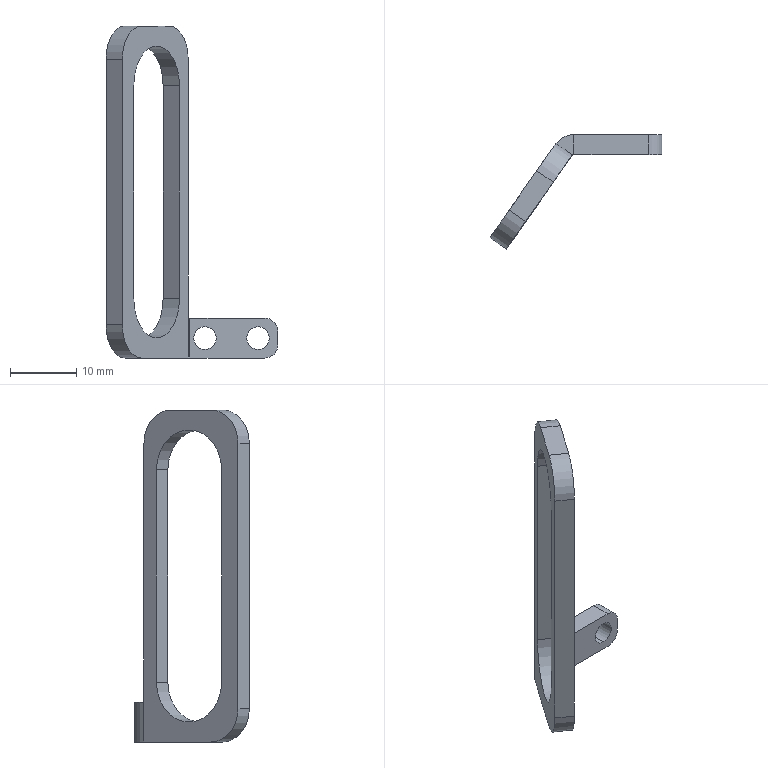Part | SolidWorks | features Fillet 2, ICE 2, EdgeFlange 1, FlatPattern 1, HoleWzd 1, SMBaseFlange 1, SheetMetal 1 | 1 solid | 28 faces | box 25.898 x 17.285 x 50 mm | volume 1263 mm3 | plane 15 | cylinder 13 | commonest cylinder face diameters 3.4 x4 10 x3 4 x2 12 x2 0.6 x1 6.6 x1
STEP:
#1=CARTESIAN_POINT('',(12.,0.,4.7));
#2=VERTEX_POINT('',#1);
#3=CARTESIAN_POINT('',(12.,0.,1.3));
#4=VERTEX_POINT('',#3);
#5=CARTESIAN_POINT('',(12.,0.,3.));
#6=DIRECTION('',(0.,-1.,0.));
#7=DIRECTION('',(0.,0.,-1.));
#8=AXIS2_PLACEMENT_3D('',#5,#6,#7);
#9=CIRCLE('',#8,1.7);
#10=EDGE_CURVE('',#2,#4,#9,.T.);
#11=ORIENTED_EDGE('',*,*,#10,.F.);
#12=CARTESIAN_POINT('',(12.,-3.,4.7));
#13=VERTEX_POINT('',#12);
#14=CARTESIAN_POINT('',(12.,-3.,4.7));
#15=DIRECTION('',(0.,-1.,0.));
#16=VECTOR('',#15,1000.);
#17=LINE('',#14,#16);
#18=EDGE_CURVE('',#2,#13,#17,.T.);
#19=ORIENTED_EDGE('',*,*,#18,.T.);
#20=CARTESIAN_POINT('',(12.,-3.,1.3));
#21=VERTEX_POINT('',#20);
#22=CARTESIAN_POINT('',(12.,-3.,3.));
#23=DIRECTION('',(0.,-1.,0.));
#24=DIRECTION('',(0.,0.,-1.));
#25=AXIS2_PLACEMENT_3D('',#22,#23,#24);
#26=CIRCLE('',#25,1.7);
#27=EDGE_CURVE('',#13,#21,#26,.T.);
#28=ORIENTED_EDGE('',*,*,#27,.T.);
#29=CARTESIAN_POINT('',(12.,-3.,1.3));
#30=DIRECTION('',(0.,-1.,0.));
#31=VECTOR('',#30,1000.);
#32=LINE('',#29,#31);
#33=EDGE_CURVE('',#4,#21,#32,.T.);
#34=ORIENTED_EDGE('',*,*,#33,.F.);
#35=EDGE_LOOP('',(#11,#19,#28,#34));
#36=FACE_OUTER_BOUND('',#35,.T.);
#37=CARTESIAN_POINT('',(12.,-3.,3.));
#38=DIRECTION('',(0.,-1.,0.));
#39=DIRECTION('',(0.,0.,-1.));
#40=AXIS2_PLACEMENT_3D('',#37,#38,#39);
#41=CYLINDRICAL_SURFACE('',#40,1.7);
#42=ADVANCED_FACE('',(#36),#41,.F.);
#43=CARTESIAN_POINT('',(4.,0.,4.7));
#44=VERTEX_POINT('',#43);
#45=CARTESIAN_POINT('',(4.,0.,1.3));
#46=VERTEX_POINT('',#45);
#47=CARTESIAN_POINT('',(4.,0.,3.));
#48=DIRECTION('',(0.,-1.,0.));
#49=DIRECTION('',(0.,0.,-1.));
#50=AXIS2_PLACEMENT_3D('',#47,#48,#49);
#51=CIRCLE('',#50,1.7);
#52=EDGE_CURVE('',#44,#46,#51,.T.);
#53=ORIENTED_EDGE('',*,*,#52,.F.);
#54=CARTESIAN_POINT('',(4.,-3.,4.7));
#55=VERTEX_POINT('',#54);
#56=CARTESIAN_POINT('',(4.,-3.,4.7));
#57=DIRECTION('',(0.,-1.,0.));
#58=VECTOR('',#57,1000.);
#59=LINE('',#56,#58);
#60=EDGE_CURVE('',#44,#55,#59,.T.);
#61=ORIENTED_EDGE('',*,*,#60,.T.);
#62=CARTESIAN_POINT('',(4.,-3.,1.3));
#63=VERTEX_POINT('',#62);
#64=CARTESIAN_POINT('',(4.,-3.,3.));
#65=DIRECTION('',(0.,-1.,0.));
#66=DIRECTION('',(0.,0.,-1.));
#67=AXIS2_PLACEMENT_3D('',#64,#65,#66);
#68=CIRCLE('',#67,1.7);
#69=EDGE_CURVE('',#55,#63,#68,.T.);
#70=ORIENTED_EDGE('',*,*,#69,.T.);
#71=CARTESIAN_POINT('',(4.,-3.,1.3));
#72=DIRECTION('',(0.,-1.,0.));
#73=VECTOR('',#72,1000.);
#74=LINE('',#71,#73);
#75=EDGE_CURVE('',#46,#63,#74,.T.);
#76=ORIENTED_EDGE('',*,*,#75,.F.);
#77=EDGE_LOOP('',(#53,#61,#70,#76));
#78=FACE_OUTER_BOUND('',#77,.T.);
#79=CARTESIAN_POINT('',(4.,-3.,3.));
#80=DIRECTION('',(0.,-1.,0.));
#81=DIRECTION('',(0.,0.,-1.));
#82=AXIS2_PLACEMENT_3D('',#79,#80,#81);
#83=CYLINDRICAL_SURFACE('',#82,1.7);
#84=ADVANCED_FACE('',(#78),#83,.F.);
#85=CARTESIAN_POINT('',(12.,-3.,3.));
#86=DIRECTION('',(0.,-1.,0.));
#87=DIRECTION('',(0.,0.,-1.));
#88=AXIS2_PLACEMENT_3D('',#85,#86,#87);
#89=CIRCLE('',#88,1.7);
#90=EDGE_CURVE('',#21,#13,#89,.T.);
#91=ORIENTED_EDGE('',*,*,#90,.F.);
#92=ORIENTED_EDGE('',*,*,#27,.F.);
#93=EDGE_LOOP('',(#91,#92));
#94=FACE_BOUND('',#93,.T.);
#95=CARTESIAN_POINT('',(4.,-3.,3.));
#96=DIRECTION('',(0.,-1.,0.));
#97=DIRECTION('',(0.,0.,-1.));
#98=AXIS2_PLACEMENT_3D('',#95,#96,#97);
#99=CIRCLE('',#98,1.7);
#100=EDGE_CURVE('',#63,#55,#99,.T.);
#101=ORIENTED_EDGE('',*,*,#100,.F.);
#102=ORIENTED_EDGE('',*,*,#69,.F.);
#103=EDGE_LOOP('',(#101,#102));
#104=FACE_BOUND('',#103,.T.);
#105=CARTESIAN_POINT('',(1.718,-3.,0.));
#106=VERTEX_POINT('',#105);
#107=CARTESIAN_POINT('',(13.,-3.,0.));
#108=VERTEX_POINT('',#107);
#109=CARTESIAN_POINT('',(0.,-3.,0.));
#110=DIRECTION('',(1.,0.,0.));
#111=VECTOR('',#110,1000.);
#112=LINE('',#109,#111);
#113=EDGE_CURVE('',#106,#108,#112,.T.);
#114=ORIENTED_EDGE('',*,*,#113,.T.);
#115=CARTESIAN_POINT('',(15.,-3.,2.));
#116=VERTEX_POINT('',#115);
#117=CARTESIAN_POINT('',(13.,-3.,2.));
#118=DIRECTION('',(0.,-1.,0.));
#119=DIRECTION('',(0.,0.,1.));
#120=AXIS2_PLACEMENT_3D('',#117,#118,#119);
#121=CIRCLE('',#120,2.);
#122=EDGE_CURVE('',#108,#116,#121,.T.);
#123=ORIENTED_EDGE('',*,*,#122,.T.);
#124=CARTESIAN_POINT('',(15.,-3.,4.));
#125=VERTEX_POINT('',#124);
#126=CARTESIAN_POINT('',(15.,-3.,6.));
#127=DIRECTION('',(0.,0.,-1.));
#128=VECTOR('',#127,1000.);
#129=LINE('',#126,#128);
#130=EDGE_CURVE('',#125,#116,#129,.T.);
#131=ORIENTED_EDGE('',*,*,#130,.F.);
#132=CARTESIAN_POINT('',(13.,-3.,6.));
#133=VERTEX_POINT('',#132);
#134=CARTESIAN_POINT('',(13.,-3.,4.));
#135=DIRECTION('',(0.,-1.,0.));
#136=DIRECTION('',(0.,0.,1.));
#137=AXIS2_PLACEMENT_3D('',#134,#135,#136);
#138=CIRCLE('',#137,2.);
#139=EDGE_CURVE('',#125,#133,#138,.T.);
#140=ORIENTED_EDGE('',*,*,#139,.T.);
#141=CARTESIAN_POINT('',(1.718,-3.,6.));
#142=VERTEX_POINT('',#141);
#143=CARTESIAN_POINT('',(0.,-3.,6.));
#144=DIRECTION('',(1.,0.,0.));
#145=VECTOR('',#144,1000.);
#146=LINE('',#143,#145);
#147=EDGE_CURVE('',#142,#133,#146,.T.);
#148=ORIENTED_EDGE('',*,*,#147,.F.);
#149=CARTESIAN_POINT('',(1.718,-3.,0.));
#150=DIRECTION('',(0.,0.,1.));
#151=VECTOR('',#150,1000.);
#152=LINE('',#149,#151);
#153=EDGE_CURVE('',#106,#142,#152,.T.);
#154=ORIENTED_EDGE('',*,*,#153,.F.);
#155=EDGE_LOOP('',(#114,#123,#131,#140,#148,#154));
#156=FACE_OUTER_BOUND('',#155,.T.);
#157=CARTESIAN_POINT('',(0.,-3.,6.));
#158=DIRECTION('',(0.,1.,0.));
#159=DIRECTION('',(0.,0.,1.));
#160=AXIS2_PLACEMENT_3D('',#157,#158,#159);
#161=PLANE('',#160);
#162=ADVANCED_FACE('',(#94,#104,#156),#161,.F.);
#163=CARTESIAN_POINT('',(12.,0.,3.));
#164=DIRECTION('',(0.,-1.,0.));
#165=DIRECTION('',(0.,0.,-1.));
#166=AXIS2_PLACEMENT_3D('',#163,#164,#165);
#167=CIRCLE('',#166,1.7);
#168=EDGE_CURVE('',#4,#2,#167,.T.);
#169=ORIENTED_EDGE('',*,*,#168,.T.);
#170=ORIENTED_EDGE('',*,*,#10,.T.);
#171=EDGE_LOOP('',(#169,#170));
#172=FACE_BOUND('',#171,.T.);
#173=CARTESIAN_POINT('',(4.,0.,3.));
#174=DIRECTION('',(0.,-1.,0.));
#175=DIRECTION('',(0.,0.,-1.));
#176=AXIS2_PLACEMENT_3D('',#173,#174,#175);
#177=CIRCLE('',#176,1.7);
#178=EDGE_CURVE('',#46,#44,#177,.T.);
#179=ORIENTED_EDGE('',*,*,#178,.T.);
#180=ORIENTED_EDGE('',*,*,#52,.T.);
#181=EDGE_LOOP('',(#179,#180));
#182=FACE_BOUND('',#181,.T.);
#183=CARTESIAN_POINT('',(15.,0.,4.));
#184=VERTEX_POINT('',#183);
#185=CARTESIAN_POINT('',(15.,0.,2.));
#186=VERTEX_POINT('',#185);
#187=CARTESIAN_POINT('',(15.,0.,6.));
#188=DIRECTION('',(0.,0.,-1.));
#189=VECTOR('',#188,1000.);
#190=LINE('',#187,#189);
#191=EDGE_CURVE('',#184,#186,#190,.T.);
#192=ORIENTED_EDGE('',*,*,#191,.T.);
#193=CARTESIAN_POINT('',(13.,0.,0.));
#194=VERTEX_POINT('',#193);
#195=CARTESIAN_POINT('',(13.,0.,2.));
#196=DIRECTION('',(0.,1.,0.));
#197=DIRECTION('',(0.,0.,1.));
#198=AXIS2_PLACEMENT_3D('',#195,#196,#197);
#199=CIRCLE('',#198,2.);
#200=EDGE_CURVE('',#186,#194,#199,.T.);
#201=ORIENTED_EDGE('',*,*,#200,.T.);
#202=CARTESIAN_POINT('',(1.718,0.,0.));
#203=VERTEX_POINT('',#202);
#204=CARTESIAN_POINT('',(0.,0.,0.));
#205=DIRECTION('',(1.,0.,0.));
#206=VECTOR('',#205,1000.);
#207=LINE('',#204,#206);
#208=EDGE_CURVE('',#203,#194,#207,.T.);
#209=ORIENTED_EDGE('',*,*,#208,.F.);
#210=CARTESIAN_POINT('',(1.718,0.,6.));
#211=VERTEX_POINT('',#210);
#212=CARTESIAN_POINT('',(1.718,0.,0.));
#213=DIRECTION('',(0.,0.,1.));
#214=VECTOR('',#213,1000.);
#215=LINE('',#212,#214);
#216=EDGE_CURVE('',#203,#211,#215,.T.);
#217=ORIENTED_EDGE('',*,*,#216,.T.);
#218=CARTESIAN_POINT('',(13.,0.,6.));
#219=VERTEX_POINT('',#218);
#220=CARTESIAN_POINT('',(0.,0.,6.));
#221=DIRECTION('',(1.,0.,0.));
#222=VECTOR('',#221,1000.);
#223=LINE('',#220,#222);
#224=EDGE_CURVE('',#211,#219,#223,.T.);
#225=ORIENTED_EDGE('',*,*,#224,.T.);
#226=CARTESIAN_POINT('',(13.,0.,4.));
#227=DIRECTION('',(0.,1.,0.));
#228=DIRECTION('',(0.,0.,1.));
#229=AXIS2_PLACEMENT_3D('',#226,#227,#228);
#230=CIRCLE('',#229,2.);
#231=EDGE_CURVE('',#219,#184,#230,.T.);
#232=ORIENTED_EDGE('',*,*,#231,.T.);
#233=EDGE_LOOP('',(#192,#201,#209,#217,#225,#232));
#234=FACE_OUTER_BOUND('',#233,.T.);
#235=CARTESIAN_POINT('',(0.,0.,6.));
#236=DIRECTION('',(0.,1.,0.));
#237=DIRECTION('',(0.,0.,1.));
#238=AXIS2_PLACEMENT_3D('',#235,#236,#237);
#239=PLANE('',#238);
#240=ADVANCED_FACE('',(#172,#182,#234),#239,.T.);
#241=ORIENTED_EDGE('',*,*,#147,.T.);
#242=CARTESIAN_POINT('',(13.,0.,6.));
#243=DIRECTION('',(0.,1.,0.));
#244=VECTOR('',#243,1000.);
#245=LINE('',#242,#244);
#246=EDGE_CURVE('',#133,#219,#245,.T.);
#247=ORIENTED_EDGE('',*,*,#246,.T.);
#248=ORIENTED_EDGE('',*,*,#224,.F.);
#249=CARTESIAN_POINT('',(1.718,-3.,6.));
#250=DIRECTION('',(0.,1.,0.));
#251=VECTOR('',#250,1000.);
#252=LINE('',#249,#251);
#253=EDGE_CURVE('',#142,#211,#252,.T.);
#254=ORIENTED_EDGE('',*,*,#253,.F.);
#255=EDGE_LOOP('',(#241,#247,#248,#254));
#256=FACE_OUTER_BOUND('',#255,.T.);
#257=CARTESIAN_POINT('',(0.,0.,6.));
#258=DIRECTION('',(0.,0.,-1.));
#259=DIRECTION('',(-1.,0.,0.));
#260=AXIS2_PLACEMENT_3D('',#257,#258,#259);
#261=PLANE('',#260);
#262=ADVANCED_FACE('',(#256),#261,.F.);
#263=ORIENTED_EDGE('',*,*,#208,.T.);
#264=CARTESIAN_POINT('',(13.,0.,0.));
#265=DIRECTION('',(0.,-1.,0.));
#266=VECTOR('',#265,1000.);
#267=LINE('',#264,#266);
#268=EDGE_CURVE('',#194,#108,#267,.T.);
#269=ORIENTED_EDGE('',*,*,#268,.T.);
#270=ORIENTED_EDGE('',*,*,#113,.F.);
#271=CARTESIAN_POINT('',(1.718,-3.,0.));
#272=DIRECTION('',(0.,1.,0.));
#273=VECTOR('',#272,1000.);
#274=LINE('',#271,#273);
#275=EDGE_CURVE('',#106,#203,#274,.T.);
#276=ORIENTED_EDGE('',*,*,#275,.T.);
#277=EDGE_LOOP('',(#263,#269,#270,#276));
#278=FACE_OUTER_BOUND('',#277,.T.);
#279=CARTESIAN_POINT('',(0.,0.,0.));
#280=DIRECTION('',(0.,0.,-1.));
#281=DIRECTION('',(-1.,0.,0.));
#282=AXIS2_PLACEMENT_3D('',#279,#280,#281);
#283=PLANE('',#282);
#284=ADVANCED_FACE('',(#278),#283,.T.);
#285=ORIENTED_EDGE('',*,*,#130,.T.);
#286=CARTESIAN_POINT('',(15.,0.,2.));
#287=DIRECTION('',(0.,1.,0.));
#288=VECTOR('',#287,1000.);
#289=LINE('',#286,#288);
#290=EDGE_CURVE('',#116,#186,#289,.T.);
#291=ORIENTED_EDGE('',*,*,#290,.T.);
#292=ORIENTED_EDGE('',*,*,#191,.F.);
#293=CARTESIAN_POINT('',(15.,-3.,4.));
#294=DIRECTION('',(0.,-1.,0.));
#295=VECTOR('',#294,1000.);
#296=LINE('',#293,#295);
#297=EDGE_CURVE('',#184,#125,#296,.T.);
#298=ORIENTED_EDGE('',*,*,#297,.T.);
#299=EDGE_LOOP('',(#285,#291,#292,#298));
#300=FACE_OUTER_BOUND('',#299,.T.);
#301=CARTESIAN_POINT('',(15.,0.,6.));
#302=DIRECTION('',(1.,0.,0.));
#303=DIRECTION('',(0.,0.,-1.));
#304=AXIS2_PLACEMENT_3D('',#301,#302,#303);
#305=PLANE('',#304);
#306=ADVANCED_FACE('',(#300),#305,.T.);
#307=CARTESIAN_POINT('',(1.472,-3.128,6.));
#308=VERTEX_POINT('',#307);
#309=CARTESIAN_POINT('',(-0.9853,-1.407,6.));
#310=VERTEX_POINT('',#309);
#311=CARTESIAN_POINT('',(1.472,-3.128,6.));
#312=DIRECTION('',(-0.8192,0.5736,0.));
#313=VECTOR('',#312,1000.);
#314=LINE('',#311,#313);
#315=EDGE_CURVE('',#308,#310,#314,.T.);
#316=ORIENTED_EDGE('',*,*,#315,.F.);
#317=CARTESIAN_POINT('',(1.718,-3.3,6.));
#318=DIRECTION('',(0.,0.,1.));
#319=DIRECTION('',(-1.,0.,0.));
#320=AXIS2_PLACEMENT_3D('',#317,#318,#319);
#321=CIRCLE('',#320,0.3);
#322=EDGE_CURVE('',#142,#308,#321,.T.);
#323=ORIENTED_EDGE('',*,*,#322,.F.);
#324=ORIENTED_EDGE('',*,*,#253,.T.);
#325=CARTESIAN_POINT('',(1.718,-3.3,6.));
#326=DIRECTION('',(0.,0.,1.));
#327=DIRECTION('',(-1.,0.,0.));
#328=AXIS2_PLACEMENT_3D('',#325,#326,#327);
#329=CIRCLE('',#328,3.3);
#330=EDGE_CURVE('',#211,#310,#329,.T.);
#331=ORIENTED_EDGE('',*,*,#330,.T.);
#332=EDGE_LOOP('',(#316,#323,#324,#331));
#333=FACE_OUTER_BOUND('',#332,.T.);
#334=CARTESIAN_POINT('',(1.718,-3.3,6.));
#335=DIRECTION('',(0.,0.,1.));
#336=DIRECTION('',(1.,0.,0.));
#337=AXIS2_PLACEMENT_3D('',#334,#335,#336);
#338=PLANE('',#337);
#339=ADVANCED_FACE('',(#333),#338,.T.);
#340=CARTESIAN_POINT('',(1.472,-3.128,0.));
#341=VERTEX_POINT('',#340);
#342=CARTESIAN_POINT('',(1.718,-3.3,0.));
#343=DIRECTION('',(0.,0.,-1.));
#344=DIRECTION('',(-1.,0.,0.));
#345=AXIS2_PLACEMENT_3D('',#342,#343,#344);
#346=CIRCLE('',#345,0.3);
#347=EDGE_CURVE('',#341,#106,#346,.T.);
#348=ORIENTED_EDGE('',*,*,#347,.F.);
#349=CARTESIAN_POINT('',(-0.9853,-1.407,0.));
#350=VERTEX_POINT('',#349);
#351=CARTESIAN_POINT('',(1.472,-3.128,0.));
#352=DIRECTION('',(-0.8192,0.5736,0.));
#353=VECTOR('',#352,1000.);
#354=LINE('',#351,#353);
#355=EDGE_CURVE('',#341,#350,#354,.T.);
#356=ORIENTED_EDGE('',*,*,#355,.T.);
#357=CARTESIAN_POINT('',(1.718,-3.3,0.));
#358=DIRECTION('',(0.,0.,-1.));
#359=DIRECTION('',(-1.,0.,0.));
#360=AXIS2_PLACEMENT_3D('',#357,#358,#359);
#361=CIRCLE('',#360,3.3);
#362=EDGE_CURVE('',#350,#203,#361,.T.);
#363=ORIENTED_EDGE('',*,*,#362,.T.);
#364=ORIENTED_EDGE('',*,*,#275,.F.);
#365=EDGE_LOOP('',(#348,#356,#363,#364));
#366=FACE_OUTER_BOUND('',#365,.T.);
#367=CARTESIAN_POINT('',(1.718,-3.3,0.));
#368=DIRECTION('',(0.,0.,1.));
#369=DIRECTION('',(1.,0.,0.));
#370=AXIS2_PLACEMENT_3D('',#367,#368,#369);
#371=PLANE('',#370);
#372=ADVANCED_FACE('',(#366),#371,.F.);
#373=ORIENTED_EDGE('',*,*,#216,.F.);
#374=ORIENTED_EDGE('',*,*,#362,.F.);
#375=CARTESIAN_POINT('',(-0.9853,-1.407,50.));
#376=DIRECTION('',(0.,0.,1.));
#377=VECTOR('',#376,1000.);
#378=LINE('',#375,#377);
#379=EDGE_CURVE('',#350,#310,#378,.T.);
#380=ORIENTED_EDGE('',*,*,#379,.T.);
#381=ORIENTED_EDGE('',*,*,#330,.F.);
#382=EDGE_LOOP('',(#373,#374,#380,#381));
#383=FACE_OUTER_BOUND('',#382,.T.);
#384=CARTESIAN_POINT('',(1.718,-3.3,0.));
#385=DIRECTION('',(0.,0.,-1.));
#386=DIRECTION('',(-0.8192,0.5736,0.));
#387=AXIS2_PLACEMENT_3D('',#384,#385,#386);
#388=CYLINDRICAL_SURFACE('',#387,3.3);
#389=ADVANCED_FACE('',(#383),#388,.T.);
#390=ORIENTED_EDGE('',*,*,#153,.T.);
#391=ORIENTED_EDGE('',*,*,#322,.T.);
#392=CARTESIAN_POINT('',(1.472,-3.128,0.));
#393=DIRECTION('',(0.,0.,-1.));
#394=VECTOR('',#393,1000.);
#395=LINE('',#392,#394);
#396=EDGE_CURVE('',#308,#341,#395,.T.);
#397=ORIENTED_EDGE('',*,*,#396,.T.);
#398=ORIENTED_EDGE('',*,*,#347,.T.);
#399=EDGE_LOOP('',(#390,#391,#397,#398));
#400=FACE_OUTER_BOUND('',#399,.T.);
#401=CARTESIAN_POINT('',(1.718,-3.3,0.));
#402=DIRECTION('',(0.,0.,-1.));
#403=DIRECTION('',(-0.8192,0.5736,0.));
#404=AXIS2_PLACEMENT_3D('',#401,#402,#403);
#405=CYLINDRICAL_SURFACE('',#404,0.3);
#406=ADVANCED_FACE('',(#400),#405,.F.);
#407=CARTESIAN_POINT('',(-5.573,-13.189,50.));
#408=VERTEX_POINT('',#407);
#409=CARTESIAN_POINT('',(-1.396,-7.224,50.));
#410=VERTEX_POINT('',#409);
#411=CARTESIAN_POINT('',(1.562,-3.,50.));
#412=DIRECTION('',(0.5736,0.8192,0.));
#413=VECTOR('',#412,1000.);
#414=LINE('',#411,#413);
#415=EDGE_CURVE('',#408,#410,#414,.T.);
#416=ORIENTED_EDGE('',*,*,#415,.T.);
#417=CARTESIAN_POINT('',(-3.853,-5.503,50.));
#418=VERTEX_POINT('',#417);
#419=CARTESIAN_POINT('',(-3.853,-5.503,50.));
#420=DIRECTION('',(-0.8192,0.5736,0.));
#421=VECTOR('',#420,1000.);
#422=LINE('',#419,#421);
#423=EDGE_CURVE('',#410,#418,#422,.T.);
#424=ORIENTED_EDGE('',*,*,#423,.T.);
#425=CARTESIAN_POINT('',(-8.03,-11.468,50.));
#426=VERTEX_POINT('',#425);
#427=CARTESIAN_POINT('',(0.5138,0.7338,50.));
#428=DIRECTION('',(0.5736,0.8192,0.));
#429=VECTOR('',#428,1000.);
#430=LINE('',#427,#429);
#431=EDGE_CURVE('',#426,#418,#430,.T.);
#432=ORIENTED_EDGE('',*,*,#431,.F.);
#433=CARTESIAN_POINT('',(-8.03,-11.468,50.));
#434=DIRECTION('',(0.8192,-0.5736,0.));
#435=VECTOR('',#434,1000.);
#436=LINE('',#433,#435);
#437=EDGE_CURVE('',#426,#408,#436,.T.);
#438=ORIENTED_EDGE('',*,*,#437,.T.);
#439=EDGE_LOOP('',(#416,#424,#432,#438));
#440=FACE_OUTER_BOUND('',#439,.T.);
#441=CARTESIAN_POINT('',(-0.8958,-1.279,50.));
#442=DIRECTION('',(0.,0.,-1.));
#443=DIRECTION('',(-1.,0.,0.));
#444=AXIS2_PLACEMENT_3D('',#441,#442,#443);
#445=PLANE('',#444);
#446=ADVANCED_FACE('',(#440),#445,.F.);
#447=CARTESIAN_POINT('',(-5.573,-13.189,0.));
#448=VERTEX_POINT('',#447);
#449=CARTESIAN_POINT('',(-8.44,-17.285,0.));
#450=DIRECTION('',(-0.5736,-0.8192,0.));
#451=VECTOR('',#450,1000.);
#452=LINE('',#449,#451);
#453=EDGE_CURVE('',#341,#448,#452,.T.);
#454=ORIENTED_EDGE('',*,*,#453,.T.);
#455=CARTESIAN_POINT('',(-8.03,-11.468,0.));
#456=VERTEX_POINT('',#455);
#457=CARTESIAN_POINT('',(-8.03,-11.468,0.));
#458=DIRECTION('',(-0.8192,0.5736,0.));
#459=VECTOR('',#458,1000.);
#460=LINE('',#457,#459);
#461=EDGE_CURVE('',#448,#456,#460,.T.);
#462=ORIENTED_EDGE('',*,*,#461,.T.);
#463=CARTESIAN_POINT('',(0.5138,0.7338,0.));
#464=DIRECTION('',(-0.5736,-0.8192,0.));
#465=VECTOR('',#464,1000.);
#466=LINE('',#463,#465);
#467=EDGE_CURVE('',#350,#456,#466,.T.);
#468=ORIENTED_EDGE('',*,*,#467,.F.);
#469=ORIENTED_EDGE('',*,*,#355,.F.);
#470=EDGE_LOOP('',(#454,#462,#468,#469));
#471=FACE_OUTER_BOUND('',#470,.T.);
#472=CARTESIAN_POINT('',(-10.898,-15.564,0.));
#473=DIRECTION('',(0.,0.,1.));
#474=DIRECTION('',(1.,0.,0.));
#475=AXIS2_PLACEMENT_3D('',#472,#473,#474);
#476=PLANE('',#475);
#477=ADVANCED_FACE('',(#471),#476,.F.);
#478=CARTESIAN_POINT('',(-2.294,-3.277,9.));
#479=VERTEX_POINT('',#478);
#480=CARTESIAN_POINT('',(-2.294,-3.277,41.));
#481=VERTEX_POINT('',#480);
#482=CARTESIAN_POINT('',(-2.294,-3.277,0.));
#483=DIRECTION('',(0.,0.,1.));
#484=VECTOR('',#483,1000.);
#485=LINE('',#482,#484);
#486=EDGE_CURVE('',#479,#481,#485,.T.);
#487=ORIENTED_EDGE('',*,*,#486,.T.);
#488=CARTESIAN_POINT('',(-9.177,-13.106,41.));
#489=VERTEX_POINT('',#488);
#490=CARTESIAN_POINT('',(-5.736,-8.192,41.));
#491=DIRECTION('',(0.8192,-0.5736,0.));
#492=DIRECTION('',(0.5736,0.8192,0.));
#493=AXIS2_PLACEMENT_3D('',#490,#491,#492);
#494=CIRCLE('',#493,6.);
#495=EDGE_CURVE('',#481,#489,#494,.T.);
#496=ORIENTED_EDGE('',*,*,#495,.T.);
#497=CARTESIAN_POINT('',(-9.177,-13.106,9.));
#498=VERTEX_POINT('',#497);
#499=CARTESIAN_POINT('',(-9.177,-13.106,0.));
#500=DIRECTION('',(0.,0.,-1.));
#501=VECTOR('',#500,1000.);
#502=LINE('',#499,#501);
#503=EDGE_CURVE('',#489,#498,#502,.T.);
#504=ORIENTED_EDGE('',*,*,#503,.T.);
#505=CARTESIAN_POINT('',(-5.736,-8.192,9.));
#506=DIRECTION('',(0.8192,-0.5736,0.));
#507=DIRECTION('',(0.5736,0.8192,0.));
#508=AXIS2_PLACEMENT_3D('',#505,#506,#507);
#509=CIRCLE('',#508,6.);
#510=EDGE_CURVE('',#498,#479,#509,.T.);
#511=ORIENTED_EDGE('',*,*,#510,.T.);
#512=EDGE_LOOP('',(#487,#496,#504,#511));
#513=FACE_BOUND('',#512,.T.);
#514=ORIENTED_EDGE('',*,*,#431,.T.);
#515=CARTESIAN_POINT('',(-0.9853,-1.407,45.));
#516=VERTEX_POINT('',#515);
#517=CARTESIAN_POINT('',(-3.853,-5.503,45.));
#518=DIRECTION('',(-0.8192,0.5736,0.));
#519=DIRECTION('',(0.5736,0.8192,0.));
#520=AXIS2_PLACEMENT_3D('',#517,#518,#519);
#521=CIRCLE('',#520,5.);
#522=EDGE_CURVE('',#418,#516,#521,.T.);
#523=ORIENTED_EDGE('',*,*,#522,.T.);
#524=CARTESIAN_POINT('',(-0.9853,-1.407,50.));
#525=DIRECTION('',(0.,0.,1.));
#526=VECTOR('',#525,1000.);
#527=LINE('',#524,#526);
#528=EDGE_CURVE('',#310,#516,#527,.T.);
#529=ORIENTED_EDGE('',*,*,#528,.F.);
#530=ORIENTED_EDGE('',*,*,#379,.F.);
#531=ORIENTED_EDGE('',*,*,#467,.T.);
#532=CARTESIAN_POINT('',(-10.898,-15.564,5.));
#533=VERTEX_POINT('',#532);
#534=CARTESIAN_POINT('',(-8.03,-11.468,5.));
#535=DIRECTION('',(-0.8192,0.5736,0.));
#536=DIRECTION('',(0.5736,0.8192,0.));
#537=AXIS2_PLACEMENT_3D('',#534,#535,#536);
#538=CIRCLE('',#537,5.);
#539=EDGE_CURVE('',#456,#533,#538,.T.);
#540=ORIENTED_EDGE('',*,*,#539,.T.);
#541=CARTESIAN_POINT('',(-10.898,-15.564,45.));
#542=VERTEX_POINT('',#541);
#543=CARTESIAN_POINT('',(-10.898,-15.564,0.));
#544=DIRECTION('',(0.,0.,1.));
#545=VECTOR('',#544,1000.);
#546=LINE('',#543,#545);
#547=EDGE_CURVE('',#533,#542,#546,.T.);
#548=ORIENTED_EDGE('',*,*,#547,.T.);
#549=CARTESIAN_POINT('',(-8.03,-11.468,45.));
#550=DIRECTION('',(-0.8192,0.5736,0.));
#551=DIRECTION('',(0.5736,0.8192,0.));
#552=AXIS2_PLACEMENT_3D('',#549,#550,#551);
#553=CIRCLE('',#552,5.);
#554=EDGE_CURVE('',#542,#426,#553,.T.);
#555=ORIENTED_EDGE('',*,*,#554,.T.);
#556=EDGE_LOOP('',(#514,#523,#529,#530,#531,#540,#548,#555));
#557=FACE_OUTER_BOUND('',#556,.T.);
#558=CARTESIAN_POINT('',(0.5138,0.7338,0.));
#559=DIRECTION('',(0.8192,-0.5736,0.));
#560=DIRECTION('',(0.5736,0.8192,0.));
#561=AXIS2_PLACEMENT_3D('',#558,#559,#560);
#562=PLANE('',#561);
#563=ADVANCED_FACE('',(#513,#557),#562,.F.);
#564=CARTESIAN_POINT('',(0.1632,-4.997,41.));
#565=VERTEX_POINT('',#564);
#566=CARTESIAN_POINT('',(-6.72,-14.827,41.));
#567=VERTEX_POINT('',#566);
#568=CARTESIAN_POINT('',(-3.278,-9.912,41.));
#569=DIRECTION('',(0.8192,-0.5736,0.));
#570=DIRECTION('',(0.5736,0.8192,0.));
#571=AXIS2_PLACEMENT_3D('',#568,#569,#570);
#572=CIRCLE('',#571,6.);
#573=EDGE_CURVE('',#565,#567,#572,.T.);
#574=ORIENTED_EDGE('',*,*,#573,.F.);
#575=CARTESIAN_POINT('',(0.1632,-4.997,9.));
#576=VERTEX_POINT('',#575);
#577=CARTESIAN_POINT('',(0.1632,-4.997,41.));
#578=DIRECTION('',(0.,0.,1.));
#579=VECTOR('',#578,1000.);
#580=LINE('',#577,#579);
#581=EDGE_CURVE('',#576,#565,#580,.T.);
#582=ORIENTED_EDGE('',*,*,#581,.F.);
#583=CARTESIAN_POINT('',(-6.72,-14.827,9.));
#584=VERTEX_POINT('',#583);
#585=CARTESIAN_POINT('',(-3.278,-9.912,9.));
#586=DIRECTION('',(0.8192,-0.5736,0.));
#587=DIRECTION('',(0.5736,0.8192,0.));
#588=AXIS2_PLACEMENT_3D('',#585,#586,#587);
#589=CIRCLE('',#588,6.);
#590=EDGE_CURVE('',#584,#576,#589,.T.);
#591=ORIENTED_EDGE('',*,*,#590,.F.);
#592=CARTESIAN_POINT('',(-6.72,-14.827,41.));
#593=DIRECTION('',(0.,0.,-1.));
#594=VECTOR('',#593,1000.);
#595=LINE('',#592,#594);
#596=EDGE_CURVE('',#567,#584,#595,.T.);
#597=ORIENTED_EDGE('',*,*,#596,.F.);
#598=EDGE_LOOP('',(#574,#582,#591,#597));
#599=FACE_BOUND('',#598,.T.);
#600=CARTESIAN_POINT('',(1.472,-3.128,45.));
#601=VERTEX_POINT('',#600);
#602=CARTESIAN_POINT('',(1.472,-3.128,50.));
#603=DIRECTION('',(0.,0.,-1.));
#604=VECTOR('',#603,1000.);
#605=LINE('',#602,#604);
#606=EDGE_CURVE('',#601,#308,#605,.T.);
#607=ORIENTED_EDGE('',*,*,#606,.F.);
#608=CARTESIAN_POINT('',(-1.396,-7.224,45.));
#609=DIRECTION('',(0.8192,-0.5736,0.));
#610=DIRECTION('',(0.5736,0.8192,0.));
#611=AXIS2_PLACEMENT_3D('',#608,#609,#610);
#612=CIRCLE('',#611,5.);
#613=EDGE_CURVE('',#601,#410,#612,.T.);
#614=ORIENTED_EDGE('',*,*,#613,.T.);
#615=ORIENTED_EDGE('',*,*,#415,.F.);
#616=CARTESIAN_POINT('',(-8.44,-17.285,45.));
#617=VERTEX_POINT('',#616);
#618=CARTESIAN_POINT('',(-5.573,-13.189,45.));
#619=DIRECTION('',(0.8192,-0.5736,0.));
#620=DIRECTION('',(0.5736,0.8192,0.));
#621=AXIS2_PLACEMENT_3D('',#618,#619,#620);
#622=CIRCLE('',#621,5.);
#623=EDGE_CURVE('',#408,#617,#622,.T.);
#624=ORIENTED_EDGE('',*,*,#623,.T.);
#625=CARTESIAN_POINT('',(-8.44,-17.285,5.));
#626=VERTEX_POINT('',#625);
#627=CARTESIAN_POINT('',(-8.44,-17.285,50.));
#628=DIRECTION('',(0.,0.,1.));
#629=VECTOR('',#628,1000.);
#630=LINE('',#627,#629);
#631=EDGE_CURVE('',#626,#617,#630,.T.);
#632=ORIENTED_EDGE('',*,*,#631,.F.);
#633=CARTESIAN_POINT('',(-5.573,-13.189,5.));
#634=DIRECTION('',(0.8192,-0.5736,0.));
#635=DIRECTION('',(0.5736,0.8192,0.));
#636=AXIS2_PLACEMENT_3D('',#633,#634,#635);
#637=CIRCLE('',#636,5.);
#638=EDGE_CURVE('',#626,#448,#637,.T.);
#639=ORIENTED_EDGE('',*,*,#638,.T.);
#640=ORIENTED_EDGE('',*,*,#453,.F.);
#641=ORIENTED_EDGE('',*,*,#396,.F.);
#642=EDGE_LOOP('',(#607,#614,#615,#624,#632,#639,#640,#641));
#643=FACE_OUTER_BOUND('',#642,.T.);
#644=CARTESIAN_POINT('',(2.971,-0.987,0.));
#645=DIRECTION('',(0.8192,-0.5736,0.));
#646=DIRECTION('',(0.5736,0.8192,0.));
#647=AXIS2_PLACEMENT_3D('',#644,#645,#646);
#648=PLANE('',#647);
#649=ADVANCED_FACE('',(#599,#643),#648,.T.);
#650=ORIENTED_EDGE('',*,*,#631,.T.);
#651=CARTESIAN_POINT('',(-10.898,-15.564,45.));
#652=DIRECTION('',(-0.8192,0.5736,0.));
#653=VECTOR('',#652,1000.);
#654=LINE('',#651,#653);
#655=EDGE_CURVE('',#617,#542,#654,.T.);
#656=ORIENTED_EDGE('',*,*,#655,.T.);
#657=ORIENTED_EDGE('',*,*,#547,.F.);
#658=CARTESIAN_POINT('',(-10.898,-15.564,5.));
#659=DIRECTION('',(0.8192,-0.5736,0.));
#660=VECTOR('',#659,1000.);
#661=LINE('',#658,#660);
#662=EDGE_CURVE('',#533,#626,#661,.T.);
#663=ORIENTED_EDGE('',*,*,#662,.T.);
#664=EDGE_LOOP('',(#650,#656,#657,#663));
#665=FACE_OUTER_BOUND('',#664,.T.);
#666=CARTESIAN_POINT('',(-10.898,-15.564,50.));
#667=DIRECTION('',(0.5736,0.8192,0.));
#668=DIRECTION('',(-0.8192,0.5736,0.));
#669=AXIS2_PLACEMENT_3D('',#666,#667,#668);
#670=PLANE('',#669);
#671=ADVANCED_FACE('',(#665),#670,.F.);
#672=ORIENTED_EDGE('',*,*,#528,.T.);
#673=CARTESIAN_POINT('',(1.472,-3.128,45.));
#674=DIRECTION('',(0.8192,-0.5736,0.));
#675=VECTOR('',#674,1000.);
#676=LINE('',#673,#675);
#677=EDGE_CURVE('',#516,#601,#676,.T.);
#678=ORIENTED_EDGE('',*,*,#677,.T.);
#679=ORIENTED_EDGE('',*,*,#606,.T.);
#680=ORIENTED_EDGE('',*,*,#315,.T.);
#681=EDGE_LOOP('',(#672,#678,#679,#680));
#682=FACE_OUTER_BOUND('',#681,.T.);
#683=CARTESIAN_POINT('',(1.472,-3.128,50.));
#684=DIRECTION('',(0.5736,0.8192,0.));
#685=DIRECTION('',(-0.8192,0.5736,0.));
#686=AXIS2_PLACEMENT_3D('',#683,#684,#685);
#687=PLANE('',#686);
#688=ADVANCED_FACE('',(#682),#687,.T.);
#689=CARTESIAN_POINT('',(-9.607,1.844,41.));
#690=DIRECTION('',(0.8192,-0.5736,0.));
#691=VECTOR('',#690,1000.);
#692=LINE('',#689,#691);
#693=EDGE_CURVE('',#481,#565,#692,.T.);
#694=ORIENTED_EDGE('',*,*,#693,.T.);
#695=ORIENTED_EDGE('',*,*,#573,.T.);
#696=CARTESIAN_POINT('',(-16.49,-7.986,41.));
#697=DIRECTION('',(0.8192,-0.5736,0.));
#698=VECTOR('',#697,1000.);
#699=LINE('',#696,#698);
#700=EDGE_CURVE('',#489,#567,#699,.T.);
#701=ORIENTED_EDGE('',*,*,#700,.F.);
#702=ORIENTED_EDGE('',*,*,#495,.F.);
#703=EDGE_LOOP('',(#694,#695,#701,#702));
#704=FACE_OUTER_BOUND('',#703,.T.);
#705=CARTESIAN_POINT('',(-13.048,-3.071,41.));
#706=DIRECTION('',(0.8192,-0.5736,0.));
#707=DIRECTION('',(0.5736,0.8192,0.));
#708=AXIS2_PLACEMENT_3D('',#705,#706,#707);
#709=CYLINDRICAL_SURFACE('',#708,6.);
#710=ADVANCED_FACE('',(#704),#709,.F.);
#711=CARTESIAN_POINT('',(-9.607,1.844,9.));
#712=DIRECTION('',(0.8192,-0.5736,0.));
#713=VECTOR('',#712,1000.);
#714=LINE('',#711,#713);
#715=EDGE_CURVE('',#479,#576,#714,.T.);
#716=ORIENTED_EDGE('',*,*,#715,.T.);
#717=ORIENTED_EDGE('',*,*,#581,.T.);
#718=ORIENTED_EDGE('',*,*,#693,.F.);
#719=ORIENTED_EDGE('',*,*,#486,.F.);
#720=EDGE_LOOP('',(#716,#717,#718,#719));
#721=FACE_OUTER_BOUND('',#720,.T.);
#722=CARTESIAN_POINT('',(-9.607,1.844,41.));
#723=DIRECTION('',(0.5736,0.8192,0.));
#724=DIRECTION('',(-0.8192,0.5736,0.));
#725=AXIS2_PLACEMENT_3D('',#722,#723,#724);
#726=PLANE('',#725);
#727=ADVANCED_FACE('',(#721),#726,.F.);
#728=CARTESIAN_POINT('',(-16.49,-7.986,9.));
#729=DIRECTION('',(0.8192,-0.5736,0.));
#730=VECTOR('',#729,1000.);
#731=LINE('',#728,#730);
#732=EDGE_CURVE('',#498,#584,#731,.T.);
#733=ORIENTED_EDGE('',*,*,#732,.T.);
#734=ORIENTED_EDGE('',*,*,#590,.T.);
#735=ORIENTED_EDGE('',*,*,#715,.F.);
#736=ORIENTED_EDGE('',*,*,#510,.F.);
#737=EDGE_LOOP('',(#733,#734,#735,#736));
#738=FACE_OUTER_BOUND('',#737,.T.);
#739=CARTESIAN_POINT('',(-13.048,-3.071,9.));
#740=DIRECTION('',(0.8192,-0.5736,0.));
#741=DIRECTION('',(0.5736,0.8192,0.));
#742=AXIS2_PLACEMENT_3D('',#739,#740,#741);
#743=CYLINDRICAL_SURFACE('',#742,6.);
#744=ADVANCED_FACE('',(#738),#743,.F.);
#745=ORIENTED_EDGE('',*,*,#700,.T.);
#746=ORIENTED_EDGE('',*,*,#596,.T.);
#747=ORIENTED_EDGE('',*,*,#732,.F.);
#748=ORIENTED_EDGE('',*,*,#503,.F.);
#749=EDGE_LOOP('',(#745,#746,#747,#748));
#750=FACE_OUTER_BOUND('',#749,.T.);
#751=CARTESIAN_POINT('',(-16.49,-7.986,41.));
#752=DIRECTION('',(-0.5736,-0.8192,0.));
#753=DIRECTION('',(0.8192,-0.5736,0.));
#754=AXIS2_PLACEMENT_3D('',#751,#752,#753);
#755=PLANE('',#754);
#756=ADVANCED_FACE('',(#750),#755,.F.);
#757=ORIENTED_EDGE('',*,*,#60,.F.);
#758=ORIENTED_EDGE('',*,*,#178,.F.);
#759=ORIENTED_EDGE('',*,*,#75,.T.);
#760=ORIENTED_EDGE('',*,*,#100,.T.);
#761=EDGE_LOOP('',(#757,#758,#759,#760));
#762=FACE_OUTER_BOUND('',#761,.T.);
#763=CARTESIAN_POINT('',(4.,-3.,3.));
#764=DIRECTION('',(0.,-1.,0.));
#765=DIRECTION('',(0.,0.,-1.));
#766=AXIS2_PLACEMENT_3D('',#763,#764,#765);
#767=CYLINDRICAL_SURFACE('',#766,1.7);
#768=ADVANCED_FACE('',(#762),#767,.F.);
#769=ORIENTED_EDGE('',*,*,#18,.F.);
#770=ORIENTED_EDGE('',*,*,#168,.F.);
#771=ORIENTED_EDGE('',*,*,#33,.T.);
#772=ORIENTED_EDGE('',*,*,#90,.T.);
#773=EDGE_LOOP('',(#769,#770,#771,#772));
#774=FACE_OUTER_BOUND('',#773,.T.);
#775=CARTESIAN_POINT('',(12.,-3.,3.));
#776=DIRECTION('',(0.,-1.,0.));
#777=DIRECTION('',(0.,0.,-1.));
#778=AXIS2_PLACEMENT_3D('',#775,#776,#777);
#779=CYLINDRICAL_SURFACE('',#778,1.7);
#780=ADVANCED_FACE('',(#774),#779,.F.);
#781=ORIENTED_EDGE('',*,*,#200,.F.);
#782=ORIENTED_EDGE('',*,*,#290,.F.);
#783=ORIENTED_EDGE('',*,*,#122,.F.);
#784=ORIENTED_EDGE('',*,*,#268,.F.);
#785=EDGE_LOOP('',(#781,#782,#783,#784));
#786=FACE_OUTER_BOUND('',#785,.T.);
#787=CARTESIAN_POINT('',(13.,0.,2.));
#788=DIRECTION('',(0.,-1.,0.));
#789=DIRECTION('',(0.,0.,-1.));
#790=AXIS2_PLACEMENT_3D('',#787,#788,#789);
#791=CYLINDRICAL_SURFACE('',#790,2.);
#792=ADVANCED_FACE('',(#786),#791,.T.);
#793=ORIENTED_EDGE('',*,*,#231,.F.);
#794=ORIENTED_EDGE('',*,*,#246,.F.);
#795=ORIENTED_EDGE('',*,*,#139,.F.);
#796=ORIENTED_EDGE('',*,*,#297,.F.);
#797=EDGE_LOOP('',(#793,#794,#795,#796));
#798=FACE_OUTER_BOUND('',#797,.T.);
#799=CARTESIAN_POINT('',(13.,0.,4.));
#800=DIRECTION('',(0.,1.,0.));
#801=DIRECTION('',(0.,0.,1.));
#802=AXIS2_PLACEMENT_3D('',#799,#800,#801);
#803=CYLINDRICAL_SURFACE('',#802,2.);
#804=ADVANCED_FACE('',(#798),#803,.T.);
#805=ORIENTED_EDGE('',*,*,#613,.F.);
#806=ORIENTED_EDGE('',*,*,#677,.F.);
#807=ORIENTED_EDGE('',*,*,#522,.F.);
#808=ORIENTED_EDGE('',*,*,#423,.F.);
#809=EDGE_LOOP('',(#805,#806,#807,#808));
#810=FACE_OUTER_BOUND('',#809,.T.);
#811=CARTESIAN_POINT('',(-3.853,-5.503,45.));
#812=DIRECTION('',(0.8192,-0.5736,0.));
#813=DIRECTION('',(0.5736,0.8192,0.));
#814=AXIS2_PLACEMENT_3D('',#811,#812,#813);
#815=CYLINDRICAL_SURFACE('',#814,5.);
#816=ADVANCED_FACE('',(#810),#815,.T.);
#817=ORIENTED_EDGE('',*,*,#554,.F.);
#818=ORIENTED_EDGE('',*,*,#655,.F.);
#819=ORIENTED_EDGE('',*,*,#623,.F.);
#820=ORIENTED_EDGE('',*,*,#437,.F.);
#821=EDGE_LOOP('',(#817,#818,#819,#820));
#822=FACE_OUTER_BOUND('',#821,.T.);
#823=CARTESIAN_POINT('',(-8.03,-11.468,45.));
#824=DIRECTION('',(0.8192,-0.5736,0.));
#825=DIRECTION('',(0.5736,0.8192,0.));
#826=AXIS2_PLACEMENT_3D('',#823,#824,#825);
#827=CYLINDRICAL_SURFACE('',#826,5.);
#828=ADVANCED_FACE('',(#822),#827,.T.);
#829=ORIENTED_EDGE('',*,*,#539,.F.);
#830=ORIENTED_EDGE('',*,*,#461,.F.);
#831=ORIENTED_EDGE('',*,*,#638,.F.);
#832=ORIENTED_EDGE('',*,*,#662,.F.);
#833=EDGE_LOOP('',(#829,#830,#831,#832));
#834=FACE_OUTER_BOUND('',#833,.T.);
#835=CARTESIAN_POINT('',(-8.03,-11.468,5.));
#836=DIRECTION('',(0.8192,-0.5736,0.));
#837=DIRECTION('',(0.5736,0.8192,0.));
#838=AXIS2_PLACEMENT_3D('',#835,#836,#837);
#839=CYLINDRICAL_SURFACE('',#838,5.);
#840=ADVANCED_FACE('',(#834),#839,.T.);
#841=CLOSED_SHELL('',(#42,#84,#162,#240,#262,#284,#306,#339,#372,#389,#406,#446,#477,#563,#649,#671,#688,#710,#727,#744,#756,#768,#780,#792,#804,#816,#828,#840));
#842=MANIFOLD_SOLID_BREP('',#841);
#843=CARTESIAN_POINT('',(0.,0.,0.));
#844=DIRECTION('',(0.,0.,1.));
#845=DIRECTION('',(1.,0.,0.));
#846=AXIS2_PLACEMENT_3D('',#843,#844,#845);
#847=(LENGTH_UNIT()NAMED_UNIT(*)SI_UNIT(.MILLI.,.METRE.));
#848=UNCERTAINTY_MEASURE_WITH_UNIT(LENGTH_MEASURE(0.00001),#847,'','');
#849=(NAMED_UNIT(*)PLANE_ANGLE_UNIT()SI_UNIT($,.RADIAN.));
#850=(NAMED_UNIT(*)SI_UNIT($,.STERADIAN.)SOLID_ANGLE_UNIT());
#851=(GEOMETRIC_REPRESENTATION_CONTEXT(3)GLOBAL_UNCERTAINTY_ASSIGNED_CONTEXT((#848))GLOBAL_UNIT_ASSIGNED_CONTEXT((#847,#849,#850))REPRESENTATION_CONTEXT('',''));
#852=ADVANCED_BREP_SHAPE_REPRESENTATION('',(#842,#846),#851);